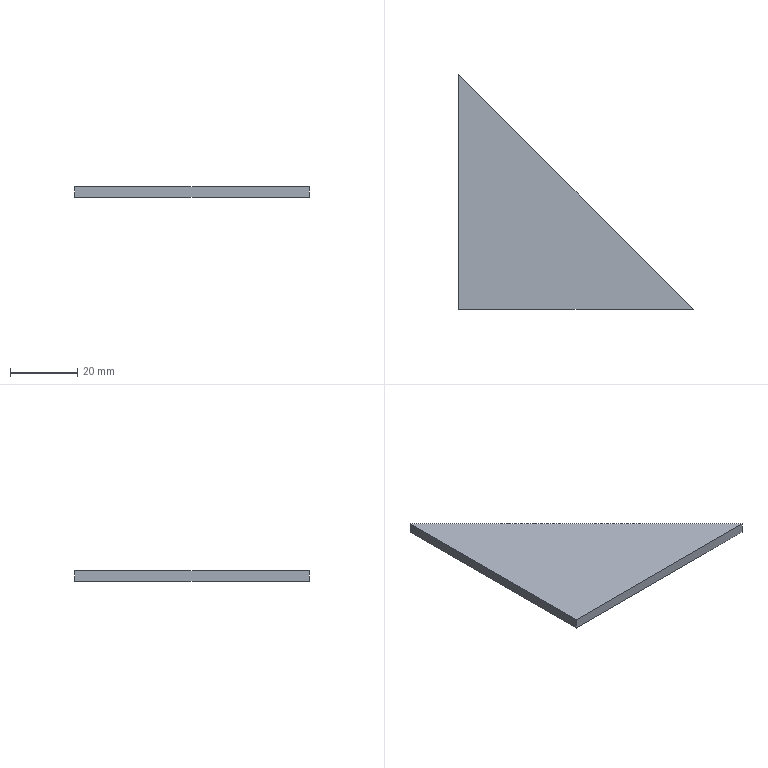Part | STEP file | 6100523 | 1 solid | 5 faces | box 70 x 70 x 3 mm | volume 7350 mm3 | plane 5
STEP:
#1=CARTESIAN_POINT('',(0.,0.,0.));
#2=DIRECTION('',(0.,0.,1.));
#3=DIRECTION('',(1.,0.,0.));
#4=AXIS2_PLACEMENT_3D('',#1,#2,#3);
#5=CARTESIAN_POINT('',(-15.009,53.935,0.));
#6=VERTEX_POINT('',#5);
#7=CARTESIAN_POINT('',(-15.009,-16.065,0.));
#8=VERTEX_POINT('',#7);
#9=CARTESIAN_POINT('',(-15.009,-16.065,0.));
#10=DIRECTION('',(0.,-1.,0.));
#11=VECTOR('',#10,1.);
#12=LINE('',#9,#11);
#13=CARTESIAN_POINT('',(-15.009,-16.065,3.));
#14=DIRECTION('',(1.,0.,0.));
#15=DIRECTION('',(0.,0.,-1.));
#16=AXIS2_PLACEMENT_3D('',#13,#14,#15);
#17=PLANE('',#16);
#18=CARTESIAN_POINT('',(3.,0.));
#19=DIRECTION('',(0.,-1.));
#20=VECTOR('',#19,1.);
#21=LINE('',#18,#20);
#22=(GEOMETRIC_REPRESENTATION_CONTEXT(2)PARAMETRIC_REPRESENTATION_CONTEXT()REPRESENTATION_CONTEXT('',''));
#23=DEFINITIONAL_REPRESENTATION('',(#21),#22);
#24=PCURVE('',#17,#23);
#25=CARTESIAN_POINT('',(-15.009,-16.065,0.));
#26=DIRECTION('',(0.,0.,1.));
#27=DIRECTION('',(1.,0.,0.));
#28=AXIS2_PLACEMENT_3D('',#25,#26,#27);
#29=PLANE('',#28);
#30=CARTESIAN_POINT('',(0.,0.));
#31=DIRECTION('',(0.,-1.));
#32=VECTOR('',#31,1.);
#33=LINE('',#30,#32);
#34=(GEOMETRIC_REPRESENTATION_CONTEXT(2)PARAMETRIC_REPRESENTATION_CONTEXT()REPRESENTATION_CONTEXT('',''));
#35=DEFINITIONAL_REPRESENTATION('',(#33),#34);
#36=PCURVE('',#29,#35);
#37=SURFACE_CURVE('',#12,(#24,#36),.PCURVE_S1.);
#38=EDGE_CURVE('',#6,#8,#37,.T.);
#39=ORIENTED_EDGE('',*,*,#38,.T.);
#40=CARTESIAN_POINT('',(-15.009,-16.065,3.));
#41=VERTEX_POINT('',#40);
#42=CARTESIAN_POINT('',(-15.009,-16.065,3.));
#43=DIRECTION('',(0.,0.,-1.));
#44=VECTOR('',#43,1.);
#45=LINE('',#42,#44);
#46=CARTESIAN_POINT('',(0.,0.));
#47=DIRECTION('',(1.,0.));
#48=VECTOR('',#47,1.);
#49=LINE('',#46,#48);
#50=(GEOMETRIC_REPRESENTATION_CONTEXT(2)PARAMETRIC_REPRESENTATION_CONTEXT()REPRESENTATION_CONTEXT('',''));
#51=DEFINITIONAL_REPRESENTATION('',(#49),#50);
#52=PCURVE('',#17,#51);
#53=CARTESIAN_POINT('',(54.991,-16.065,3.));
#54=DIRECTION('',(0.,1.,0.));
#55=DIRECTION('',(-1.,0.,0.));
#56=AXIS2_PLACEMENT_3D('',#53,#54,#55);
#57=PLANE('',#56);
#58=CARTESIAN_POINT('',(70.,0.));
#59=DIRECTION('',(0.,-1.));
#60=VECTOR('',#59,1.);
#61=LINE('',#58,#60);
#62=(GEOMETRIC_REPRESENTATION_CONTEXT(2)PARAMETRIC_REPRESENTATION_CONTEXT()REPRESENTATION_CONTEXT('',''));
#63=DEFINITIONAL_REPRESENTATION('',(#61),#62);
#64=PCURVE('',#57,#63);
#65=SURFACE_CURVE('',#45,(#52,#64),.PCURVE_S1.);
#66=EDGE_CURVE('',#41,#8,#65,.T.);
#67=ORIENTED_EDGE('',*,*,#66,.F.);
#68=CARTESIAN_POINT('',(-15.009,53.935,3.));
#69=VERTEX_POINT('',#68);
#70=CARTESIAN_POINT('',(-15.009,-16.065,3.));
#71=DIRECTION('',(0.,-1.,0.));
#72=VECTOR('',#71,1.);
#73=LINE('',#70,#72);
#74=CARTESIAN_POINT('',(0.,0.));
#75=DIRECTION('',(0.,-1.));
#76=VECTOR('',#75,1.);
#77=LINE('',#74,#76);
#78=(GEOMETRIC_REPRESENTATION_CONTEXT(2)PARAMETRIC_REPRESENTATION_CONTEXT()REPRESENTATION_CONTEXT('',''));
#79=DEFINITIONAL_REPRESENTATION('',(#77),#78);
#80=PCURVE('',#17,#79);
#81=CARTESIAN_POINT('',(-15.009,-16.065,3.));
#82=DIRECTION('',(0.,0.,1.));
#83=DIRECTION('',(1.,0.,0.));
#84=AXIS2_PLACEMENT_3D('',#81,#82,#83);
#85=PLANE('',#84);
#86=CARTESIAN_POINT('',(0.,0.));
#87=DIRECTION('',(0.,-1.));
#88=VECTOR('',#87,1.);
#89=LINE('',#86,#88);
#90=(GEOMETRIC_REPRESENTATION_CONTEXT(2)PARAMETRIC_REPRESENTATION_CONTEXT()REPRESENTATION_CONTEXT('',''));
#91=DEFINITIONAL_REPRESENTATION('',(#89),#90);
#92=PCURVE('',#85,#91);
#93=SURFACE_CURVE('',#73,(#80,#92),.PCURVE_S1.);
#94=EDGE_CURVE('',#69,#41,#93,.T.);
#95=ORIENTED_EDGE('',*,*,#94,.F.);
#96=CARTESIAN_POINT('',(-15.009,53.935,3.));
#97=DIRECTION('',(0.,0.,-1.));
#98=VECTOR('',#97,1.);
#99=LINE('',#96,#98);
#100=CARTESIAN_POINT('',(0.,70.));
#101=DIRECTION('',(1.,0.));
#102=VECTOR('',#101,1.);
#103=LINE('',#100,#102);
#104=(GEOMETRIC_REPRESENTATION_CONTEXT(2)PARAMETRIC_REPRESENTATION_CONTEXT()REPRESENTATION_CONTEXT('',''));
#105=DEFINITIONAL_REPRESENTATION('',(#103),#104);
#106=PCURVE('',#17,#105);
#107=CARTESIAN_POINT('',(-15.009,53.935,3.));
#108=DIRECTION('',(-0.7071,-0.7071,0.));
#109=DIRECTION('',(0.7071,-0.7071,0.));
#110=AXIS2_PLACEMENT_3D('',#107,#108,#109);
#111=PLANE('',#110);
#112=CARTESIAN_POINT('',(0.,0.));
#113=DIRECTION('',(0.,-1.));
#114=VECTOR('',#113,1.);
#115=LINE('',#112,#114);
#116=(GEOMETRIC_REPRESENTATION_CONTEXT(2)PARAMETRIC_REPRESENTATION_CONTEXT()REPRESENTATION_CONTEXT('',''));
#117=DEFINITIONAL_REPRESENTATION('',(#115),#116);
#118=PCURVE('',#111,#117);
#119=SURFACE_CURVE('',#99,(#106,#118),.PCURVE_S1.);
#120=EDGE_CURVE('',#69,#6,#119,.T.);
#121=ORIENTED_EDGE('',*,*,#120,.T.);
#122=EDGE_LOOP('',(#39,#67,#95,#121));
#123=FACE_BOUND('',#122,.T.);
#124=ADVANCED_FACE('',(#123),#17,.F.);
#125=CARTESIAN_POINT('',(54.991,-16.065,0.));
#126=VERTEX_POINT('',#125);
#127=CARTESIAN_POINT('',(54.991,-16.065,0.));
#128=DIRECTION('',(1.,0.,0.));
#129=VECTOR('',#128,1.);
#130=LINE('',#127,#129);
#131=CARTESIAN_POINT('',(0.,-3.));
#132=DIRECTION('',(-1.,0.));
#133=VECTOR('',#132,1.);
#134=LINE('',#131,#133);
#135=(GEOMETRIC_REPRESENTATION_CONTEXT(2)PARAMETRIC_REPRESENTATION_CONTEXT()REPRESENTATION_CONTEXT('',''));
#136=DEFINITIONAL_REPRESENTATION('',(#134),#135);
#137=PCURVE('',#57,#136);
#138=CARTESIAN_POINT('',(70.,0.));
#139=DIRECTION('',(1.,0.));
#140=VECTOR('',#139,1.);
#141=LINE('',#138,#140);
#142=(GEOMETRIC_REPRESENTATION_CONTEXT(2)PARAMETRIC_REPRESENTATION_CONTEXT()REPRESENTATION_CONTEXT('',''));
#143=DEFINITIONAL_REPRESENTATION('',(#141),#142);
#144=PCURVE('',#29,#143);
#145=SURFACE_CURVE('',#130,(#137,#144),.PCURVE_S1.);
#146=EDGE_CURVE('',#8,#126,#145,.T.);
#147=ORIENTED_EDGE('',*,*,#146,.T.);
#148=CARTESIAN_POINT('',(54.991,-16.065,3.));
#149=VERTEX_POINT('',#148);
#150=CARTESIAN_POINT('',(54.991,-16.065,3.));
#151=DIRECTION('',(0.,0.,-1.));
#152=VECTOR('',#151,1.);
#153=LINE('',#150,#152);
#154=CARTESIAN_POINT('',(0.,0.));
#155=DIRECTION('',(0.,-1.));
#156=VECTOR('',#155,1.);
#157=LINE('',#154,#156);
#158=(GEOMETRIC_REPRESENTATION_CONTEXT(2)PARAMETRIC_REPRESENTATION_CONTEXT()REPRESENTATION_CONTEXT('',''));
#159=DEFINITIONAL_REPRESENTATION('',(#157),#158);
#160=PCURVE('',#57,#159);
#161=CARTESIAN_POINT('',(98.995,0.));
#162=DIRECTION('',(0.,-1.));
#163=VECTOR('',#162,1.);
#164=LINE('',#161,#163);
#165=(GEOMETRIC_REPRESENTATION_CONTEXT(2)PARAMETRIC_REPRESENTATION_CONTEXT()REPRESENTATION_CONTEXT('',''));
#166=DEFINITIONAL_REPRESENTATION('',(#164),#165);
#167=PCURVE('',#111,#166);
#168=SURFACE_CURVE('',#153,(#160,#167),.PCURVE_S1.);
#169=EDGE_CURVE('',#149,#126,#168,.T.);
#170=ORIENTED_EDGE('',*,*,#169,.F.);
#171=CARTESIAN_POINT('',(54.991,-16.065,3.));
#172=DIRECTION('',(1.,0.,0.));
#173=VECTOR('',#172,1.);
#174=LINE('',#171,#173);
#175=CARTESIAN_POINT('',(0.,0.));
#176=DIRECTION('',(-1.,0.));
#177=VECTOR('',#176,1.);
#178=LINE('',#175,#177);
#179=(GEOMETRIC_REPRESENTATION_CONTEXT(2)PARAMETRIC_REPRESENTATION_CONTEXT()REPRESENTATION_CONTEXT('',''));
#180=DEFINITIONAL_REPRESENTATION('',(#178),#179);
#181=PCURVE('',#57,#180);
#182=CARTESIAN_POINT('',(70.,0.));
#183=DIRECTION('',(1.,0.));
#184=VECTOR('',#183,1.);
#185=LINE('',#182,#184);
#186=(GEOMETRIC_REPRESENTATION_CONTEXT(2)PARAMETRIC_REPRESENTATION_CONTEXT()REPRESENTATION_CONTEXT('',''));
#187=DEFINITIONAL_REPRESENTATION('',(#185),#186);
#188=PCURVE('',#85,#187);
#189=SURFACE_CURVE('',#174,(#181,#188),.PCURVE_S1.);
#190=EDGE_CURVE('',#41,#149,#189,.T.);
#191=ORIENTED_EDGE('',*,*,#190,.F.);
#192=ORIENTED_EDGE('',*,*,#66,.T.);
#193=EDGE_LOOP('',(#147,#170,#191,#192));
#194=FACE_BOUND('',#193,.T.);
#195=ADVANCED_FACE('',(#194),#57,.F.);
#196=CARTESIAN_POINT('',(-15.009,53.935,0.));
#197=DIRECTION('',(-0.7071,0.7071,0.));
#198=VECTOR('',#197,1.);
#199=LINE('',#196,#198);
#200=CARTESIAN_POINT('',(0.,-3.));
#201=DIRECTION('',(-1.,0.));
#202=VECTOR('',#201,1.);
#203=LINE('',#200,#202);
#204=(GEOMETRIC_REPRESENTATION_CONTEXT(2)PARAMETRIC_REPRESENTATION_CONTEXT()REPRESENTATION_CONTEXT('',''));
#205=DEFINITIONAL_REPRESENTATION('',(#203),#204);
#206=PCURVE('',#111,#205);
#207=CARTESIAN_POINT('',(0.,70.));
#208=DIRECTION('',(-0.7071,0.7071));
#209=VECTOR('',#208,1.);
#210=LINE('',#207,#209);
#211=(GEOMETRIC_REPRESENTATION_CONTEXT(2)PARAMETRIC_REPRESENTATION_CONTEXT()REPRESENTATION_CONTEXT('',''));
#212=DEFINITIONAL_REPRESENTATION('',(#210),#211);
#213=PCURVE('',#29,#212);
#214=SURFACE_CURVE('',#199,(#206,#213),.PCURVE_S1.);
#215=EDGE_CURVE('',#126,#6,#214,.T.);
#216=ORIENTED_EDGE('',*,*,#215,.T.);
#217=ORIENTED_EDGE('',*,*,#120,.F.);
#218=CARTESIAN_POINT('',(-15.009,53.935,3.));
#219=DIRECTION('',(-0.7071,0.7071,0.));
#220=VECTOR('',#219,1.);
#221=LINE('',#218,#220);
#222=CARTESIAN_POINT('',(0.,0.));
#223=DIRECTION('',(-1.,0.));
#224=VECTOR('',#223,1.);
#225=LINE('',#222,#224);
#226=(GEOMETRIC_REPRESENTATION_CONTEXT(2)PARAMETRIC_REPRESENTATION_CONTEXT()REPRESENTATION_CONTEXT('',''));
#227=DEFINITIONAL_REPRESENTATION('',(#225),#226);
#228=PCURVE('',#111,#227);
#229=CARTESIAN_POINT('',(0.,70.));
#230=DIRECTION('',(-0.7071,0.7071));
#231=VECTOR('',#230,1.);
#232=LINE('',#229,#231);
#233=(GEOMETRIC_REPRESENTATION_CONTEXT(2)PARAMETRIC_REPRESENTATION_CONTEXT()REPRESENTATION_CONTEXT('',''));
#234=DEFINITIONAL_REPRESENTATION('',(#232),#233);
#235=PCURVE('',#85,#234);
#236=SURFACE_CURVE('',#221,(#228,#235),.PCURVE_S1.);
#237=EDGE_CURVE('',#149,#69,#236,.T.);
#238=ORIENTED_EDGE('',*,*,#237,.F.);
#239=ORIENTED_EDGE('',*,*,#169,.T.);
#240=EDGE_LOOP('',(#216,#217,#238,#239));
#241=FACE_BOUND('',#240,.T.);
#242=ADVANCED_FACE('',(#241),#111,.F.);
#243=ORIENTED_EDGE('',*,*,#94,.T.);
#244=ORIENTED_EDGE('',*,*,#190,.T.);
#245=ORIENTED_EDGE('',*,*,#237,.T.);
#246=EDGE_LOOP('',(#243,#244,#245));
#247=FACE_BOUND('',#246,.T.);
#248=ADVANCED_FACE('',(#247),#85,.T.);
#249=ORIENTED_EDGE('',*,*,#38,.F.);
#250=ORIENTED_EDGE('',*,*,#215,.F.);
#251=ORIENTED_EDGE('',*,*,#146,.F.);
#252=EDGE_LOOP('',(#249,#250,#251));
#253=FACE_BOUND('',#252,.T.);
#254=ADVANCED_FACE('',(#253),#29,.F.);
#255=CLOSED_SHELL('',(#124,#195,#242,#248,#254));
#256=MANIFOLD_SOLID_BREP('',#255);
#257=(LENGTH_UNIT()NAMED_UNIT(*)SI_UNIT(.MILLI.,.METRE.));
#258=UNCERTAINTY_MEASURE_WITH_UNIT(LENGTH_MEASURE(0.0000001),#257,'','');
#259=(NAMED_UNIT(*)PLANE_ANGLE_UNIT()SI_UNIT($,.RADIAN.));
#260=(NAMED_UNIT(*)SI_UNIT($,.STERADIAN.)SOLID_ANGLE_UNIT());
#261=(GEOMETRIC_REPRESENTATION_CONTEXT(3)GLOBAL_UNCERTAINTY_ASSIGNED_CONTEXT((#258))GLOBAL_UNIT_ASSIGNED_CONTEXT((#257,#259,#260))REPRESENTATION_CONTEXT('',''));
#262=ADVANCED_BREP_SHAPE_REPRESENTATION('',(#4,#256),#261);